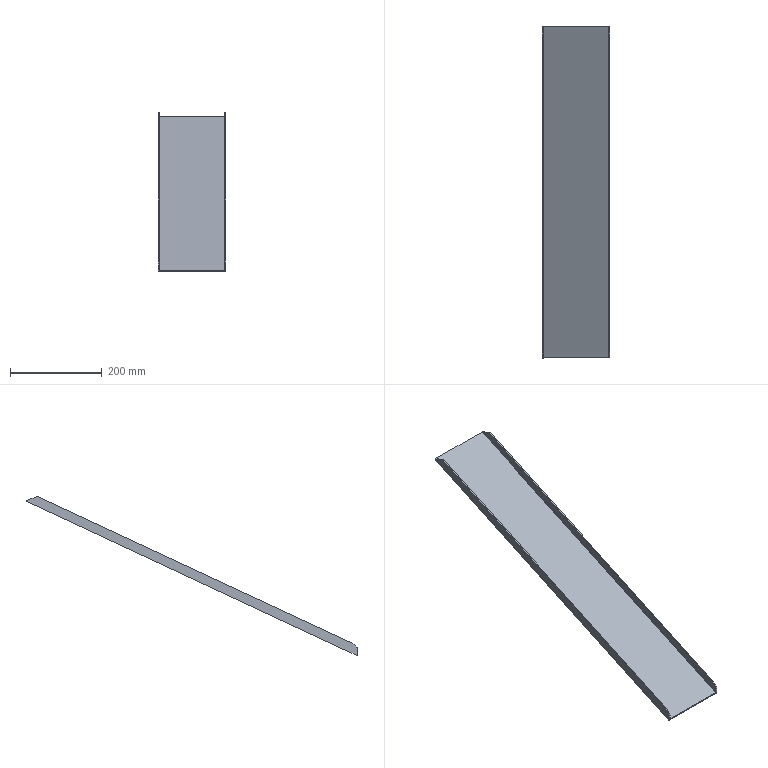Part | NX | features solid 2 | 1 solid | 16 faces | box 146.416 x 724.221 x 347.355 mm | volume 290427 mm3 | plane 9 | spline 6 | cylinder 1 | commonest cylinder face diameters 40 x1
STEP:
#1=CARTESIAN_POINT('',(-795.66,-820.,-476.696));
#2=VERTEX_POINT('',#1);
#3=CARTESIAN_POINT('',(-795.66,-820.,-478.903));
#4=VERTEX_POINT('',#3);
#5=CARTESIAN_POINT('',(-795.66,-820.,-476.696));
#6=CARTESIAN_POINT('',(-795.66,-820.,-477.432));
#7=CARTESIAN_POINT('',(-795.66,-820.,-478.167));
#8=CARTESIAN_POINT('',(-795.66,-820.,-478.902));
#9=B_SPLINE_CURVE_WITH_KNOTS('',3,(#5,#6,#7,#8),.UNSPECIFIED.,.F.,.F.,(4,4),(0.,0.002206),.UNSPECIFIED.);
#10=EDGE_CURVE('',#2,#4,#9,.T.);
#11=ORIENTED_EDGE('',*,*,#10,.F.);
#12=CARTESIAN_POINT('',(-938.,-820.,-476.696));
#13=VERTEX_POINT('',#12);
#14=CARTESIAN_POINT('',(-793.584,-820.,-476.696));
#15=DIRECTION('',(1.,0.,0.));
#16=VECTOR('',#15,1000.);
#17=LINE('',#14,#16);
#18=EDGE_CURVE('',#13,#2,#17,.T.);
#19=ORIENTED_EDGE('',*,*,#18,.F.);
#20=CARTESIAN_POINT('',(-938.,-820.,-478.903));
#21=VERTEX_POINT('',#20);
#22=CARTESIAN_POINT('',(-938.,-820.,-700.));
#23=DIRECTION('',(0.,0.,1.));
#24=VECTOR('',#23,1000.);
#25=LINE('',#22,#24);
#26=EDGE_CURVE('',#21,#13,#25,.T.);
#27=ORIENTED_EDGE('',*,*,#26,.F.);
#28=CARTESIAN_POINT('',(-793.584,-820.,-478.903));
#29=DIRECTION('',(1.,0.,0.));
#30=VECTOR('',#29,1000.);
#31=LINE('',#28,#30);
#32=EDGE_CURVE('',#21,#4,#31,.T.);
#33=ORIENTED_EDGE('',*,*,#32,.T.);
#34=EDGE_LOOP('',(#11,#19,#27,#33));
#35=FACE_BOUND('',#34,.T.);
#36=CARTESIAN_POINT('',(1065.,-820.,-700.));
#37=DIRECTION('',(0.,1.,0.));
#38=DIRECTION('',(-1.,0.,0.));
#39=AXIS2_PLACEMENT_3D('',#36,#37,#38);
#40=PLANE('',#39);
#41=ADVANCED_FACE('',(#35),#40,.F.);
#42=CARTESIAN_POINT('',(-795.584,-98.498,-140.255));
#43=VERTEX_POINT('',#42);
#44=CARTESIAN_POINT('',(-795.584,-98.499,-140.255));
#45=CARTESIAN_POINT('',(-795.661,-218.749,-196.329));
#46=CARTESIAN_POINT('',(-795.552,-459.25,-308.476));
#47=CARTESIAN_POINT('',(-795.635,-699.75,-420.623));
#48=CARTESIAN_POINT('',(-795.66,-820.,-476.696));
#49=B_SPLINE_CURVE_WITH_KNOTS('',3,(#44,#45,#46,#47,#48),.UNSPECIFIED.,.F.,.F.,(4,1,4),(0.,0.398,0.7961),.UNSPECIFIED.);
#50=EDGE_CURVE('',#43,#2,#49,.T.);
#51=ORIENTED_EDGE('',*,*,#50,.F.);
#52=CARTESIAN_POINT('',(-938.,-98.499,-140.255));
#53=VERTEX_POINT('',#52);
#54=CARTESIAN_POINT('',(-793.584,-98.499,-140.255));
#55=DIRECTION('',(-1.,0.,0.));
#56=VECTOR('',#55,1000.);
#57=LINE('',#54,#56);
#58=EDGE_CURVE('',#43,#53,#57,.T.);
#59=ORIENTED_EDGE('',*,*,#58,.T.);
#60=CARTESIAN_POINT('',(-938.,-996.354,-558.932));
#61=DIRECTION('',(0.,0.9063,0.4226));
#62=VECTOR('',#61,1000.);
#63=LINE('',#60,#62);
#64=EDGE_CURVE('',#13,#53,#63,.T.);
#65=ORIENTED_EDGE('',*,*,#64,.F.);
#66=ORIENTED_EDGE('',*,*,#18,.T.);
#67=EDGE_LOOP('',(#51,#59,#65,#66));
#68=FACE_BOUND('',#67,.T.);
#69=CARTESIAN_POINT('',(-793.584,-996.354,-558.932));
#70=DIRECTION('',(0.,0.4226,-0.9063));
#71=DIRECTION('',(-1.,0.,0.));
#72=AXIS2_PLACEMENT_3D('',#69,#70,#71);
#73=PLANE('',#72);
#74=ADVANCED_FACE('',(#68),#73,.F.);
#75=CARTESIAN_POINT('',(-795.584,-97.653,-142.067));
#76=VERTEX_POINT('',#75);
#77=CARTESIAN_POINT('',(-795.584,-97.654,-142.068));
#78=CARTESIAN_POINT('',(-795.584,-97.936,-141.463));
#79=CARTESIAN_POINT('',(-795.584,-98.217,-140.859));
#80=CARTESIAN_POINT('',(-795.584,-98.499,-140.255));
#81=B_SPLINE_CURVE_WITH_KNOTS('',3,(#77,#78,#79,#80),.UNSPECIFIED.,.F.,.F.,(4,4),(0.,1.),.UNSPECIFIED.);
#82=EDGE_CURVE('',#76,#43,#81,.T.);
#83=ORIENTED_EDGE('',*,*,#82,.F.);
#84=CARTESIAN_POINT('',(-940.,-97.654,-142.068));
#85=VERTEX_POINT('',#84);
#86=CARTESIAN_POINT('',(-793.584,-97.654,-142.068));
#87=DIRECTION('',(-1.,0.,0.));
#88=VECTOR('',#87,1000.);
#89=LINE('',#86,#88);
#90=EDGE_CURVE('',#76,#85,#89,.T.);
#91=ORIENTED_EDGE('',*,*,#90,.T.);
#92=CARTESIAN_POINT('',(-940.,-98.499,-140.255));
#93=VERTEX_POINT('',#92);
#94=CARTESIAN_POINT('',(-940.,-98.499,-140.255));
#95=DIRECTION('',(0.,0.4226,-0.9063));
#96=VECTOR('',#95,1000.);
#97=LINE('',#94,#96);
#98=EDGE_CURVE('',#93,#85,#97,.T.);
#99=ORIENTED_EDGE('',*,*,#98,.F.);
#100=CARTESIAN_POINT('',(-940.,-98.499,-140.255));
#101=DIRECTION('',(-1.,0.,0.));
#102=VECTOR('',#101,1000.);
#103=LINE('',#100,#102);
#104=EDGE_CURVE('',#93,#53,#103,.F.);
#105=ORIENTED_EDGE('',*,*,#104,.T.);
#106=ORIENTED_EDGE('',*,*,#58,.F.);
#107=EDGE_LOOP('',(#83,#91,#99,#105,#106));
#108=FACE_BOUND('',#107,.T.);
#109=CARTESIAN_POINT('',(-793.584,-98.499,-140.255));
#110=DIRECTION('',(0.,-0.9063,-0.4226));
#111=DIRECTION('',(0.,0.4226,-0.9063));
#112=AXIS2_PLACEMENT_3D('',#109,#110,#111);
#113=PLANE('',#112);
#114=ADVANCED_FACE('',(#108),#113,.F.);
#115=CARTESIAN_POINT('',(-793.66,-820.,-478.903));
#116=VERTEX_POINT('',#115);
#117=CARTESIAN_POINT('',(-793.584,-97.654,-142.068));
#118=VERTEX_POINT('',#117);
#119=CARTESIAN_POINT('',(-793.66,-820.,-478.903));
#120=CARTESIAN_POINT('',(-793.635,-699.609,-422.764));
#121=CARTESIAN_POINT('',(-793.552,-458.827,-310.485));
#122=CARTESIAN_POINT('',(-793.661,-218.045,-198.207));
#123=CARTESIAN_POINT('',(-793.584,-97.654,-142.068));
#124=B_SPLINE_CURVE_WITH_KNOTS('',3,(#119,#120,#121,#122,#123),.UNSPECIFIED.,.F.,.F.,(4,1,4),(0.,0.3985,0.797),.UNSPECIFIED.);
#125=EDGE_CURVE('',#116,#118,#124,.T.);
#126=ORIENTED_EDGE('',*,*,#125,.T.);
#127=CARTESIAN_POINT('',(-793.584,-98.499,-140.255));
#128=VERTEX_POINT('',#127);
#129=CARTESIAN_POINT('',(-793.584,-98.499,-140.255));
#130=CARTESIAN_POINT('',(-793.584,-98.217,-140.859));
#131=CARTESIAN_POINT('',(-793.584,-97.936,-141.463));
#132=CARTESIAN_POINT('',(-793.584,-97.654,-142.068));
#133=B_SPLINE_CURVE_WITH_KNOTS('',3,(#129,#130,#131,#132),.UNSPECIFIED.,.F.,.F.,(4,4),(0.,1.),.UNSPECIFIED.);
#134=EDGE_CURVE('',#118,#128,#133,.F.);
#135=ORIENTED_EDGE('',*,*,#134,.T.);
#136=CARTESIAN_POINT('',(-793.66,-820.,-476.696));
#137=VERTEX_POINT('',#136);
#138=CARTESIAN_POINT('',(-793.584,-98.499,-140.255));
#139=CARTESIAN_POINT('',(-793.586,-101.89,-141.836));
#140=CARTESIAN_POINT('',(-793.59,-108.28,-144.816));
#141=CARTESIAN_POINT('',(-793.595,-116.688,-148.736));
#142=CARTESIAN_POINT('',(-793.6,-123.917,-152.107));
#143=CARTESIAN_POINT('',(-793.603,-129.968,-154.929));
#144=CARTESIAN_POINT('',(-793.605,-134.029,-156.823));
#145=CARTESIAN_POINT('',(-793.607,-136.689,-158.063));
#146=CARTESIAN_POINT('',(-793.608,-138.389,-158.856));
#147=CARTESIAN_POINT('',(-793.608,-139.561,-159.402));
#148=CARTESIAN_POINT('',(-793.609,-140.351,-159.771));
#149=CARTESIAN_POINT('',(-793.609,-140.87,-160.013));
#150=CARTESIAN_POINT('',(-793.609,-141.315,-160.22));
#151=CARTESIAN_POINT('',(-793.609,-141.625,-160.365));
#152=CARTESIAN_POINT('',(-793.609,-141.835,-160.463));
#153=CARTESIAN_POINT('',(-793.609,-141.976,-160.528));
#154=CARTESIAN_POINT('',(-793.609,-142.076,-160.575));
#155=CARTESIAN_POINT('',(-793.609,-142.15,-160.609));
#156=CARTESIAN_POINT('',(-793.609,-142.185,-160.626));
#157=CARTESIAN_POINT('',(-793.609,-142.226,-160.645));
#158=CARTESIAN_POINT('',(-793.609,-142.216,-160.641));
#159=CARTESIAN_POINT('',(-793.609,-142.642,-160.839));
#160=CARTESIAN_POINT('',(-793.609,-143.054,-161.031));
#161=CARTESIAN_POINT('',(-793.608,-143.617,-161.294));
#162=CARTESIAN_POINT('',(-793.608,-144.479,-161.696));
#163=CARTESIAN_POINT('',(-793.608,-145.546,-162.193));
#164=CARTESIAN_POINT('',(-793.607,-147.207,-162.968));
#165=CARTESIAN_POINT('',(-793.606,-149.208,-163.901));
#166=CARTESIAN_POINT('',(-793.605,-152.244,-165.317));
#167=CARTESIAN_POINT('',(-793.603,-155.733,-166.943));
#168=CARTESIAN_POINT('',(-793.602,-159.426,-168.665));
#169=CARTESIAN_POINT('',(-793.601,-162.626,-170.158));
#170=CARTESIAN_POINT('',(-793.6,-165.334,-171.421));
#171=CARTESIAN_POINT('',(-793.599,-167.549,-172.454));
#172=CARTESIAN_POINT('',(-793.598,-169.272,-173.257));
#173=CARTESIAN_POINT('',(-793.598,-170.297,-173.735));
#174=CARTESIAN_POINT('',(-793.598,-170.871,-174.003));
#175=CARTESIAN_POINT('',(-793.598,-171.176,-174.145));
#176=CARTESIAN_POINT('',(-793.598,-171.321,-174.213));
#177=CARTESIAN_POINT('',(-793.598,-171.365,-174.233));
#178=CARTESIAN_POINT('',(-793.598,-171.406,-174.252));
#179=CARTESIAN_POINT('',(-793.597,-171.346,-174.224));
#180=CARTESIAN_POINT('',(-793.598,-171.617,-174.35));
#181=CARTESIAN_POINT('',(-793.598,-171.941,-174.501));
#182=CARTESIAN_POINT('',(-793.599,-172.461,-174.744));
#183=CARTESIAN_POINT('',(-793.6,-173.361,-175.164));
#184=CARTESIAN_POINT('',(-793.601,-174.494,-175.692));
#185=CARTESIAN_POINT('',(-793.602,-175.851,-176.325));
#186=CARTESIAN_POINT('',(-793.603,-177.66,-177.168));
#187=CARTESIAN_POINT('',(-793.605,-179.922,-178.223));
#188=CARTESIAN_POINT('',(-793.606,-182.636,-179.489));
#189=CARTESIAN_POINT('',(-793.608,-186.255,-181.176));
#190=CARTESIAN_POINT('',(-793.609,-189.874,-182.864));
#191=CARTESIAN_POINT('',(-793.609,-193.492,-184.551));
#192=CARTESIAN_POINT('',(-793.608,-195.754,-185.606));
#193=CARTESIAN_POINT('',(-793.608,-197.563,-186.449));
#194=CARTESIAN_POINT('',(-793.607,-198.696,-186.977));
#195=CARTESIAN_POINT('',(-793.607,-199.484,-187.345));
#196=CARTESIAN_POINT('',(-793.607,-199.941,-187.558));
#197=CARTESIAN_POINT('',(-793.607,-200.267,-187.71));
#198=CARTESIAN_POINT('',(-793.606,-200.592,-187.862));
#199=CARTESIAN_POINT('',(-793.606,-200.551,-187.843));
#200=CARTESIAN_POINT('',(-793.606,-200.568,-187.851));
#201=CARTESIAN_POINT('',(-793.606,-200.563,-187.848));
#202=CARTESIAN_POINT('',(-793.606,-200.596,-187.863));
#203=CARTESIAN_POINT('',(-793.606,-200.64,-187.884));
#204=CARTESIAN_POINT('',(-793.606,-200.706,-187.915));
#205=CARTESIAN_POINT('',(-793.606,-200.817,-187.967));
#206=CARTESIAN_POINT('',(-793.606,-201.001,-188.052));
#207=CARTESIAN_POINT('',(-793.606,-201.293,-188.188));
#208=CARTESIAN_POINT('',(-793.606,-201.657,-188.358));
#209=CARTESIAN_POINT('',(-793.606,-202.238,-188.629));
#210=CARTESIAN_POINT('',(-793.606,-203.144,-189.052));
#211=CARTESIAN_POINT('',(-793.606,-204.977,-189.906));
#212=CARTESIAN_POINT('',(-793.606,-207.987,-191.31));
#213=CARTESIAN_POINT('',(-793.606,-212.748,-193.53));
#214=CARTESIAN_POINT('',(-793.606,-218.659,-196.286));
#215=CARTESIAN_POINT('',(-793.605,-225.72,-199.579));
#216=CARTESIAN_POINT('',(-793.605,-233.93,-203.408));
#217=CARTESIAN_POINT('',(-793.605,-246.41,-209.227));
#218=CARTESIAN_POINT('',(-793.604,-261.19,-216.119));
#219=CARTESIAN_POINT('',(-793.604,-278.269,-224.083));
#220=CARTESIAN_POINT('',(-793.603,-292.228,-230.592));
#221=CARTESIAN_POINT('',(-793.603,-307.337,-237.637));
#222=CARTESIAN_POINT('',(-793.602,-323.595,-245.219));
#223=CARTESIAN_POINT('',(-793.602,-338.102,-251.983));
#224=CARTESIAN_POINT('',(-793.601,-350.282,-257.663));
#225=CARTESIAN_POINT('',(-793.601,-359.704,-262.057));
#226=CARTESIAN_POINT('',(-793.6,-369.414,-266.585));
#227=CARTESIAN_POINT('',(-793.6,-377.745,-270.47));
#228=CARTESIAN_POINT('',(-793.6,-384.554,-273.645));
#229=CARTESIAN_POINT('',(-793.6,-389.732,-276.059));
#230=CARTESIAN_POINT('',(-793.6,-394.107,-278.099));
#231=CARTESIAN_POINT('',(-793.6,-397.644,-279.749));
#232=CARTESIAN_POINT('',(-793.599,-399.868,-280.785));
#233=CARTESIAN_POINT('',(-793.599,-401.659,-281.621));
#234=CARTESIAN_POINT('',(-793.599,-402.775,-282.141));
#235=CARTESIAN_POINT('',(-793.599,-403.687,-282.567));
#236=CARTESIAN_POINT('',(-793.599,-404.218,-282.814));
#237=CARTESIAN_POINT('',(-793.599,-404.736,-283.056));
#238=CARTESIAN_POINT('',(-793.599,-404.8,-283.085));
#239=CARTESIAN_POINT('',(-793.599,-405.124,-283.236));
#240=CARTESIAN_POINT('',(-793.599,-405.476,-283.401));
#241=CARTESIAN_POINT('',(-793.599,-406.103,-283.693));
#242=CARTESIAN_POINT('',(-793.599,-406.868,-284.05));
#243=CARTESIAN_POINT('',(-793.599,-407.799,-284.484));
#244=CARTESIAN_POINT('',(-793.599,-409.042,-285.064));
#245=CARTESIAN_POINT('',(-793.599,-411.233,-286.085));
#246=CARTESIAN_POINT('',(-793.599,-414.401,-287.562));
#247=CARTESIAN_POINT('',(-793.599,-418.265,-289.364));
#248=CARTESIAN_POINT('',(-793.599,-422.191,-291.195));
#249=CARTESIAN_POINT('',(-793.599,-427.509,-293.675));
#250=CARTESIAN_POINT('',(-793.599,-434.313,-296.847));
#251=CARTESIAN_POINT('',(-793.599,-442.726,-300.771));
#252=CARTESIAN_POINT('',(-793.6,-454.276,-306.157));
#253=CARTESIAN_POINT('',(-793.601,-469.337,-313.179));
#254=CARTESIAN_POINT('',(-793.602,-488.406,-322.072));
#255=CARTESIAN_POINT('',(-793.604,-508.473,-331.429));
#256=CARTESIAN_POINT('',(-793.607,-529.536,-341.251));
#257=CARTESIAN_POINT('',(-793.61,-558.949,-354.966));
#258=CARTESIAN_POINT('',(-793.616,-598.208,-373.273));
#259=CARTESIAN_POINT('',(-793.624,-640.79,-393.129));
#260=CARTESIAN_POINT('',(-793.631,-676.85,-409.944));
#261=CARTESIAN_POINT('',(-793.635,-700.215,-420.84));
#262=CARTESIAN_POINT('',(-793.639,-719.412,-429.791));
#263=CARTESIAN_POINT('',(-793.643,-738.564,-438.722));
#264=CARTESIAN_POINT('',(-793.648,-762.519,-449.893));
#265=CARTESIAN_POINT('',(-793.654,-791.259,-463.294));
#266=CARTESIAN_POINT('',(-793.658,-810.42,-472.229));
#267=CARTESIAN_POINT('',(-793.66,-820.,-476.696));
#268=B_SPLINE_CURVE_WITH_KNOTS('',3,(#138,#139,#140,#141,#142,#143,#144,#145,#146,#147,#148,#149,#150,#151,#152,#153,#154,#155,#156,#157,#158,#159,#160,#161,#162,#163,#164,#165,#166,#167,#168,#169,#170,#171,#172,#173,#174,#175,#176,#177,#178,#179,#180,#181,#182,#183,#184,#185,#186,#187,#188,#189,#190,#191,#192,#193,#194,#195,#196,#197,#198,#199,#200,#201,#202,#203,#204,#205,#206,#207,#208,#209,#210,#211,#212,#213,#214,#215,#216,#217,#218,#219,#220,#221,#222,#223,#224,#225,#226,#227,#228,#229,#230,#231,#232,#233,#234,#235,#236,#237,#238,#239,#240,#241,#242,#243,#244,#245,#246,#247,#248,#249,#250,#251,#252,#253,#254,#255,#256,#257,#258,#259,#260,#261,#262,#263,#264,#265,#266,#267),.UNSPECIFIED.,.F.,.F.,(4,1,1,1,1,1,1,1,1,1,1,1,1,1,1,1,1,1,1,1,1,1,1,1,1,1,1,1,1,1,1,1,1,1,1,1,1,1,1,1,1,1,1,1,1,1,1,1,1,1,1,1,1,1,1,1,1,1,1,1,1,1,1,1,1,1,1,1,1,1,1,1,1,1,1,1,1,1,1,1,1,1,1,1,1,1,1,1,1,1,1,1,1,1,1,1,1,1,1,1,1,1,1,1,1,1,1,1,1,1,1,1,1,1,1,1,1,1,1,1,1,1,1,1,1,1,1,4),(0.,0.008865,0.01773,0.02659,0.03546,0.04432,0.04876,0.05319,0.05762,0.05984,0.06205,0.06427,0.06648,0.06759,0.0687,0.06981,0.07036,0.07092,0.07119,0.07147,0.07175,0.07202,0.07258,0.07313,0.07424,0.07535,0.07757,0.07978,0.08421,0.08865,0.09308,0.09751,0.1019,0.1064,0.1108,0.113,0.1152,0.1175,0.118,0.1186,0.1191,0.1194,0.1197,0.1208,0.1219,0.1241,0.1263,0.1285,0.133,0.1374,0.1418,0.1507,0.1551,0.1596,0.1618,0.164,0.1651,0.1657,0.1662,0.1668,0.167,0.1673,0.1684,0.1706,0.1729,0.1751,0.1773,0.1817,0.1862,0.1906,0.195,0.2039,0.2127,0.2305,0.2482,0.2659,0.2837,0.3014,0.3191,0.3546,0.3723,0.39,0.4078,0.4255,0.4432,0.4521,0.461,0.4698,0.4787,0.4831,0.4876,0.492,0.4942,0.4964,0.4975,0.4986,0.4992,0.4997,0.5,0.5003,0.5008,0.502,0.5031,0.5053,0.5075,0.5097,0.5141,0.523,0.5319,0.5407,0.5496,0.5673,0.5851,0.6028,0.6382,0.6737,0.7092,0.7446,0.7801,0.851,0.9219,0.9574,0.9928,1.011,1.028,1.064,1.099,1.135),.UNSPECIFIED.);
#269=EDGE_CURVE('',#128,#137,#268,.T.);
#270=ORIENTED_EDGE('',*,*,#269,.T.);
#271=CARTESIAN_POINT('',(-793.66,-820.,-476.696));
#272=CARTESIAN_POINT('',(-793.66,-820.,-477.432));
#273=CARTESIAN_POINT('',(-793.66,-820.,-478.168));
#274=CARTESIAN_POINT('',(-793.66,-820.,-478.903));
#275=B_SPLINE_CURVE_WITH_KNOTS('',3,(#271,#272,#273,#274),.UNSPECIFIED.,.F.,.F.,(4,4),(0.,1.),.UNSPECIFIED.);
#276=EDGE_CURVE('',#137,#116,#275,.T.);
#277=ORIENTED_EDGE('',*,*,#276,.T.);
#278=EDGE_LOOP('',(#126,#135,#270,#277));
#279=FACE_BOUND('',#278,.T.);
#280=CARTESIAN_POINT('',(-793.661,-826.369,-479.666));
#281=CARTESIAN_POINT('',(-793.661,-825.523,-481.479));
#282=CARTESIAN_POINT('',(-793.657,-807.075,-470.669));
#283=CARTESIAN_POINT('',(-793.657,-806.23,-472.482));
#284=CARTESIAN_POINT('',(-793.651,-778.138,-457.176));
#285=CARTESIAN_POINT('',(-793.651,-777.292,-458.988));
#286=CARTESIAN_POINT('',(-793.644,-744.368,-441.429));
#287=CARTESIAN_POINT('',(-793.644,-743.523,-443.241));
#288=CARTESIAN_POINT('',(-793.64,-725.084,-432.436));
#289=CARTESIAN_POINT('',(-793.64,-724.239,-434.249));
#290=CARTESIAN_POINT('',(-793.637,-710.586,-425.676));
#291=CARTESIAN_POINT('',(-793.637,-709.741,-427.488));
#292=CARTESIAN_POINT('',(-793.634,-696.222,-418.978));
#293=CARTESIAN_POINT('',(-793.634,-695.376,-420.79));
#294=CARTESIAN_POINT('',(-793.631,-677.447,-410.223));
#295=CARTESIAN_POINT('',(-793.631,-676.602,-412.036));
#296=CARTESIAN_POINT('',(-793.626,-654.597,-399.568));
#297=CARTESIAN_POINT('',(-793.626,-653.752,-401.38));
#298=CARTESIAN_POINT('',(-793.622,-628.193,-387.255));
#299=CARTESIAN_POINT('',(-793.622,-627.348,-389.068));
#300=CARTESIAN_POINT('',(-793.617,-602.798,-375.414));
#301=CARTESIAN_POINT('',(-793.617,-601.953,-377.226));
#302=CARTESIAN_POINT('',(-793.613,-578.415,-364.043));
#303=CARTESIAN_POINT('',(-793.613,-577.57,-365.856));
#304=CARTESIAN_POINT('',(-793.61,-555.042,-353.144));
#305=CARTESIAN_POINT('',(-793.61,-554.197,-354.957));
#306=CARTESIAN_POINT('',(-793.607,-532.68,-342.717));
#307=CARTESIAN_POINT('',(-793.607,-531.834,-344.529));
#308=CARTESIAN_POINT('',(-793.604,-511.328,-332.76));
#309=CARTESIAN_POINT('',(-793.604,-510.483,-334.573));
#310=CARTESIAN_POINT('',(-793.602,-490.987,-323.275));
#311=CARTESIAN_POINT('',(-793.602,-490.142,-325.088));
#312=CARTESIAN_POINT('',(-793.601,-474.879,-315.764));
#313=CARTESIAN_POINT('',(-793.601,-474.033,-317.576));
#314=CARTESIAN_POINT('',(-793.6,-462.497,-309.99));
#315=CARTESIAN_POINT('',(-793.6,-461.652,-311.803));
#316=CARTESIAN_POINT('',(-793.6,-453.464,-305.778));
#317=CARTESIAN_POINT('',(-793.6,-452.619,-307.59));
#318=CARTESIAN_POINT('',(-793.599,-444.683,-301.683));
#319=CARTESIAN_POINT('',(-793.599,-443.838,-303.496));
#320=CARTESIAN_POINT('',(-793.599,-436.155,-297.707));
#321=CARTESIAN_POINT('',(-793.599,-435.31,-299.519));
#322=CARTESIAN_POINT('',(-793.599,-429.259,-294.491));
#323=CARTESIAN_POINT('',(-793.599,-428.414,-296.303));
#324=CARTESIAN_POINT('',(-793.599,-423.868,-291.977));
#325=CARTESIAN_POINT('',(-793.599,-423.023,-293.79));
#326=CARTESIAN_POINT('',(-793.599,-419.889,-290.121));
#327=CARTESIAN_POINT('',(-793.599,-419.043,-291.934));
#328=CARTESIAN_POINT('',(-793.599,-416.625,-288.599));
#329=CARTESIAN_POINT('',(-793.599,-415.779,-290.412));
#330=CARTESIAN_POINT('',(-793.599,-414.045,-287.397));
#331=CARTESIAN_POINT('',(-793.599,-413.2,-289.209));
#332=CARTESIAN_POINT('',(-793.599,-412.126,-286.502));
#333=CARTESIAN_POINT('',(-793.599,-411.281,-288.314));
#334=CARTESIAN_POINT('',(-793.599,-410.223,-285.614));
#335=CARTESIAN_POINT('',(-793.599,-409.378,-287.427));
#336=CARTESIAN_POINT('',(-793.599,-408.651,-284.881));
#337=CARTESIAN_POINT('',(-793.599,-407.805,-286.694));
#338=CARTESIAN_POINT('',(-793.599,-407.4,-284.298));
#339=CARTESIAN_POINT('',(-793.599,-406.555,-286.111));
#340=CARTESIAN_POINT('',(-793.599,-406.623,-283.935));
#341=CARTESIAN_POINT('',(-793.599,-405.777,-285.748));
#342=CARTESIAN_POINT('',(-793.599,-406.001,-283.646));
#343=CARTESIAN_POINT('',(-793.599,-405.156,-285.458));
#344=CARTESIAN_POINT('',(-793.599,-405.54,-283.43));
#345=CARTESIAN_POINT('',(-793.599,-404.694,-285.243));
#346=CARTESIAN_POINT('',(-793.599,-405.144,-283.246));
#347=CARTESIAN_POINT('',(-793.599,-404.299,-285.059));
#348=CARTESIAN_POINT('',(-793.599,-404.891,-283.128));
#349=CARTESIAN_POINT('',(-793.599,-404.046,-284.94));
#350=CARTESIAN_POINT('',(-793.599,-404.733,-283.054));
#351=CARTESIAN_POINT('',(-793.599,-403.888,-284.867));
#352=CARTESIAN_POINT('',(-793.599,-404.693,-283.036));
#353=CARTESIAN_POINT('',(-793.599,-403.848,-284.848));
#354=CARTESIAN_POINT('',(-793.599,-404.42,-282.908));
#355=CARTESIAN_POINT('',(-793.599,-403.575,-284.721));
#356=CARTESIAN_POINT('',(-793.599,-404.159,-282.786));
#357=CARTESIAN_POINT('',(-793.599,-403.313,-284.599));
#358=CARTESIAN_POINT('',(-793.599,-403.696,-282.571));
#359=CARTESIAN_POINT('',(-793.599,-402.851,-284.383));
#360=CARTESIAN_POINT('',(-793.599,-402.909,-282.203));
#361=CARTESIAN_POINT('',(-793.599,-402.063,-284.016));
#362=CARTESIAN_POINT('',(-793.599,-401.776,-281.675));
#363=CARTESIAN_POINT('',(-793.599,-400.93,-283.488));
#364=CARTESIAN_POINT('',(-793.599,-400.425,-281.045));
#365=CARTESIAN_POINT('',(-793.599,-399.58,-282.858));
#366=CARTESIAN_POINT('',(-793.599,-398.629,-280.208));
#367=CARTESIAN_POINT('',(-793.599,-397.784,-282.02));
#368=CARTESIAN_POINT('',(-793.6,-396.396,-279.166));
#369=CARTESIAN_POINT('',(-793.6,-395.551,-280.979));
#370=CARTESIAN_POINT('',(-793.6,-392.847,-277.511));
#371=CARTESIAN_POINT('',(-793.6,-392.001,-279.324));
#372=CARTESIAN_POINT('',(-793.6,-388.456,-275.464));
#373=CARTESIAN_POINT('',(-793.6,-387.611,-277.277));
#374=CARTESIAN_POINT('',(-793.6,-383.26,-273.041));
#375=CARTESIAN_POINT('',(-793.6,-382.414,-274.854));
#376=CARTESIAN_POINT('',(-793.6,-378.136,-270.652));
#377=CARTESIAN_POINT('',(-793.6,-377.291,-272.465));
#378=CARTESIAN_POINT('',(-793.6,-371.402,-267.512));
#379=CARTESIAN_POINT('',(-793.6,-370.557,-269.324));
#380=CARTESIAN_POINT('',(-793.601,-363.167,-263.672));
#381=CARTESIAN_POINT('',(-793.601,-362.322,-265.484));
#382=CARTESIAN_POINT('',(-793.601,-353.576,-259.199));
#383=CARTESIAN_POINT('',(-793.601,-352.731,-261.012));
#384=CARTESIAN_POINT('',(-793.601,-344.276,-254.863));
#385=CARTESIAN_POINT('',(-793.601,-343.431,-256.675));
#386=CARTESIAN_POINT('',(-793.602,-335.268,-250.662));
#387=CARTESIAN_POINT('',(-793.602,-334.423,-252.475));
#388=CARTESIAN_POINT('',(-793.602,-323.646,-245.243));
#389=CARTESIAN_POINT('',(-793.602,-322.8,-247.055));
#390=CARTESIAN_POINT('',(-793.602,-309.846,-238.808));
#391=CARTESIAN_POINT('',(-793.602,-309.001,-240.62));
#392=CARTESIAN_POINT('',(-793.603,-294.453,-231.63));
#393=CARTESIAN_POINT('',(-793.603,-293.607,-233.442));
#394=CARTESIAN_POINT('',(-793.604,-280.225,-224.995));
#395=CARTESIAN_POINT('',(-793.604,-279.38,-226.808));
#396=CARTESIAN_POINT('',(-793.604,-262.808,-216.874));
#397=CARTESIAN_POINT('',(-793.604,-261.963,-218.686));
#398=CARTESIAN_POINT('',(-793.605,-247.723,-209.839));
#399=CARTESIAN_POINT('',(-793.605,-246.878,-211.652));
#400=CARTESIAN_POINT('',(-793.605,-234.97,-203.892));
#401=CARTESIAN_POINT('',(-793.605,-234.124,-205.705));
#402=CARTESIAN_POINT('',(-793.605,-226.57,-199.975));
#403=CARTESIAN_POINT('',(-793.605,-225.725,-201.788));
#404=CARTESIAN_POINT('',(-793.606,-219.336,-196.602));
#405=CARTESIAN_POINT('',(-793.606,-218.491,-198.415));
#406=CARTESIAN_POINT('',(-793.606,-213.268,-193.773));
#407=CARTESIAN_POINT('',(-793.606,-212.423,-195.585));
#408=CARTESIAN_POINT('',(-793.606,-208.365,-191.486));
#409=CARTESIAN_POINT('',(-793.606,-207.52,-193.299));
#410=CARTESIAN_POINT('',(-793.606,-205.251,-190.034));
#411=CARTESIAN_POINT('',(-793.606,-204.406,-191.847));
#412=CARTESIAN_POINT('',(-793.606,-203.343,-189.144));
#413=CARTESIAN_POINT('',(-793.606,-202.498,-190.957));
#414=CARTESIAN_POINT('',(-793.606,-202.203,-188.613));
#415=CARTESIAN_POINT('',(-793.606,-201.358,-190.426));
#416=CARTESIAN_POINT('',(-793.606,-201.496,-188.283));
#417=CARTESIAN_POINT('',(-793.606,-200.651,-190.096));
#418=CARTESIAN_POINT('',(-793.606,-201.076,-188.087));
#419=CARTESIAN_POINT('',(-793.606,-200.231,-189.9));
#420=CARTESIAN_POINT('',(-793.606,-200.834,-187.974));
#421=CARTESIAN_POINT('',(-793.606,-199.988,-189.787));
#422=CARTESIAN_POINT('',(-793.606,-200.694,-187.909));
#423=CARTESIAN_POINT('',(-793.606,-199.848,-189.722));
#424=CARTESIAN_POINT('',(-793.606,-200.615,-187.872));
#425=CARTESIAN_POINT('',(-793.606,-199.77,-189.685));
#426=CARTESIAN_POINT('',(-793.606,-200.588,-187.86));
#427=CARTESIAN_POINT('',(-793.606,-199.743,-189.672));
#428=CARTESIAN_POINT('',(-793.606,-200.56,-187.847));
#429=CARTESIAN_POINT('',(-793.606,-199.715,-189.659));
#430=CARTESIAN_POINT('',(-793.606,-200.581,-187.857));
#431=CARTESIAN_POINT('',(-793.606,-199.736,-189.669));
#432=CARTESIAN_POINT('',(-793.606,-200.532,-187.834));
#433=CARTESIAN_POINT('',(-793.606,-199.687,-189.646));
#434=CARTESIAN_POINT('',(-793.606,-200.578,-187.855));
#435=CARTESIAN_POINT('',(-793.606,-199.733,-189.668));
#436=CARTESIAN_POINT('',(-793.606,-200.429,-187.786));
#437=CARTESIAN_POINT('',(-793.606,-199.583,-189.598));
#438=CARTESIAN_POINT('',(-793.607,-200.251,-187.703));
#439=CARTESIAN_POINT('',(-793.607,-199.406,-189.515));
#440=CARTESIAN_POINT('',(-793.607,-199.955,-187.564));
#441=CARTESIAN_POINT('',(-793.607,-199.109,-189.377));
#442=CARTESIAN_POINT('',(-793.607,-199.278,-187.249));
#443=CARTESIAN_POINT('',(-793.607,-198.433,-189.062));
#444=CARTESIAN_POINT('',(-793.607,-198.248,-186.769));
#445=CARTESIAN_POINT('',(-793.607,-197.403,-188.581));
#446=CARTESIAN_POINT('',(-793.608,-196.883,-186.132));
#447=CARTESIAN_POINT('',(-793.608,-196.038,-187.945));
#448=CARTESIAN_POINT('',(-793.608,-195.517,-185.495));
#449=CARTESIAN_POINT('',(-793.608,-194.671,-187.308));
#450=CARTESIAN_POINT('',(-793.608,-193.695,-184.645));
#451=CARTESIAN_POINT('',(-793.608,-192.849,-186.458));
#452=CARTESIAN_POINT('',(-793.609,-191.417,-183.583));
#453=CARTESIAN_POINT('',(-793.609,-190.572,-185.396));
#454=CARTESIAN_POINT('',(-793.608,-188.684,-182.309));
#455=CARTESIAN_POINT('',(-793.608,-187.839,-184.122));
#456=CARTESIAN_POINT('',(-793.608,-185.951,-181.035));
#457=CARTESIAN_POINT('',(-793.608,-185.106,-182.847));
#458=CARTESIAN_POINT('',(-793.607,-183.219,-179.76));
#459=CARTESIAN_POINT('',(-793.607,-182.373,-181.573));
#460=CARTESIAN_POINT('',(-793.605,-180.486,-178.486));
#461=CARTESIAN_POINT('',(-793.605,-179.64,-180.299));
#462=CARTESIAN_POINT('',(-793.604,-178.208,-177.424));
#463=CARTESIAN_POINT('',(-793.604,-177.363,-179.237));
#464=CARTESIAN_POINT('',(-793.602,-176.386,-176.574));
#465=CARTESIAN_POINT('',(-793.602,-175.541,-178.387));
#466=CARTESIAN_POINT('',(-793.601,-175.02,-175.937));
#467=CARTESIAN_POINT('',(-793.601,-174.174,-177.75));
#468=CARTESIAN_POINT('',(-793.6,-173.882,-175.407));
#469=CARTESIAN_POINT('',(-793.6,-173.037,-177.219));
#470=CARTESIAN_POINT('',(-793.599,-172.969,-174.981));
#471=CARTESIAN_POINT('',(-793.599,-172.124,-176.793));
#472=CARTESIAN_POINT('',(-793.599,-172.405,-174.718));
#473=CARTESIAN_POINT('',(-793.599,-171.559,-176.53));
#474=CARTESIAN_POINT('',(-793.598,-171.939,-174.5));
#475=CARTESIAN_POINT('',(-793.598,-171.094,-176.313));
#476=CARTESIAN_POINT('',(-793.598,-171.681,-174.38));
#477=CARTESIAN_POINT('',(-793.598,-170.835,-176.193));
#478=CARTESIAN_POINT('',(-793.598,-171.399,-174.249));
#479=CARTESIAN_POINT('',(-793.598,-170.553,-176.061));
#480=CARTESIAN_POINT('',(-793.598,-171.392,-174.246));
#481=CARTESIAN_POINT('',(-793.598,-170.547,-176.058));
#482=CARTESIAN_POINT('',(-793.598,-171.374,-174.237));
#483=CARTESIAN_POINT('',(-793.598,-170.529,-176.05));
#484=CARTESIAN_POINT('',(-793.598,-171.329,-174.216));
#485=CARTESIAN_POINT('',(-793.598,-170.483,-176.029));
#486=CARTESIAN_POINT('',(-793.598,-171.214,-174.163));
#487=CARTESIAN_POINT('',(-793.598,-170.369,-175.975));
#488=CARTESIAN_POINT('',(-793.598,-170.993,-174.06));
#489=CARTESIAN_POINT('',(-793.598,-170.148,-175.872));
#490=CARTESIAN_POINT('',(-793.598,-170.474,-173.817));
#491=CARTESIAN_POINT('',(-793.598,-169.628,-175.63));
#492=CARTESIAN_POINT('',(-793.598,-169.512,-173.369));
#493=CARTESIAN_POINT('',(-793.598,-168.666,-175.181));
#494=CARTESIAN_POINT('',(-793.599,-167.858,-172.597));
#495=CARTESIAN_POINT('',(-793.599,-167.012,-174.41));
#496=CARTESIAN_POINT('',(-793.599,-165.704,-171.593));
#497=CARTESIAN_POINT('',(-793.599,-164.859,-173.406));
#498=CARTESIAN_POINT('',(-793.601,-163.052,-170.356));
#499=CARTESIAN_POINT('',(-793.601,-162.206,-172.169));
#500=CARTESIAN_POINT('',(-793.602,-159.899,-168.886));
#501=CARTESIAN_POINT('',(-793.602,-159.054,-170.699));
#502=CARTESIAN_POINT('',(-793.603,-156.856,-167.467));
#503=CARTESIAN_POINT('',(-793.603,-156.011,-169.28));
#504=CARTESIAN_POINT('',(-793.604,-154.172,-166.216));
#505=CARTESIAN_POINT('',(-793.604,-153.327,-168.028));
#506=CARTESIAN_POINT('',(-793.605,-152.034,-165.219));
#507=CARTESIAN_POINT('',(-793.605,-151.189,-167.031));
#508=CARTESIAN_POINT('',(-793.606,-149.771,-164.164));
#509=CARTESIAN_POINT('',(-793.606,-148.926,-165.976));
#510=CARTESIAN_POINT('',(-793.607,-147.782,-163.236));
#511=CARTESIAN_POINT('',(-793.607,-146.936,-165.048));
#512=CARTESIAN_POINT('',(-793.607,-146.127,-162.464));
#513=CARTESIAN_POINT('',(-793.607,-145.282,-164.277));
#514=CARTESIAN_POINT('',(-793.608,-145.068,-161.97));
#515=CARTESIAN_POINT('',(-793.608,-144.223,-163.783));
#516=CARTESIAN_POINT('',(-793.608,-144.203,-161.567));
#517=CARTESIAN_POINT('',(-793.608,-143.357,-163.38));
#518=CARTESIAN_POINT('',(-793.608,-143.553,-161.264));
#519=CARTESIAN_POINT('',(-793.608,-142.708,-163.076));
#520=CARTESIAN_POINT('',(-793.609,-142.983,-160.998));
#521=CARTESIAN_POINT('',(-793.609,-142.137,-162.811));
#522=CARTESIAN_POINT('',(-793.609,-142.572,-160.807));
#523=CARTESIAN_POINT('',(-793.609,-141.727,-162.619));
#524=CARTESIAN_POINT('',(-793.609,-142.201,-160.634));
#525=CARTESIAN_POINT('',(-793.609,-141.356,-162.446));
#526=CARTESIAN_POINT('',(-793.609,-142.233,-160.648));
#527=CARTESIAN_POINT('',(-793.609,-141.387,-162.461));
#528=CARTESIAN_POINT('',(-793.609,-142.207,-160.636));
#529=CARTESIAN_POINT('',(-793.609,-141.361,-162.449));
#530=CARTESIAN_POINT('',(-793.609,-142.186,-160.627));
#531=CARTESIAN_POINT('',(-793.609,-141.341,-162.439));
#532=CARTESIAN_POINT('',(-793.609,-142.141,-160.605));
#533=CARTESIAN_POINT('',(-793.609,-141.295,-162.418));
#534=CARTESIAN_POINT('',(-793.609,-142.087,-160.58));
#535=CARTESIAN_POINT('',(-793.609,-141.242,-162.393));
#536=CARTESIAN_POINT('',(-793.609,-142.007,-160.543));
#537=CARTESIAN_POINT('',(-793.609,-141.162,-162.356));
#538=CARTESIAN_POINT('',(-793.609,-141.897,-160.492));
#539=CARTESIAN_POINT('',(-793.609,-141.052,-162.304));
#540=CARTESIAN_POINT('',(-793.609,-141.695,-160.397));
#541=CARTESIAN_POINT('',(-793.609,-140.85,-162.21));
#542=CARTESIAN_POINT('',(-793.609,-141.396,-160.258));
#543=CARTESIAN_POINT('',(-793.609,-140.55,-162.071));
#544=CARTESIAN_POINT('',(-793.609,-140.962,-160.056));
#545=CARTESIAN_POINT('',(-793.609,-140.117,-161.868));
#546=CARTESIAN_POINT('',(-793.609,-140.454,-159.819));
#547=CARTESIAN_POINT('',(-793.609,-139.608,-161.631));
#548=CARTESIAN_POINT('',(-793.608,-139.676,-159.456));
#549=CARTESIAN_POINT('',(-793.608,-138.831,-161.269));
#550=CARTESIAN_POINT('',(-793.608,-138.518,-158.916));
#551=CARTESIAN_POINT('',(-793.608,-137.673,-160.729));
#552=CARTESIAN_POINT('',(-793.607,-136.829,-158.129));
#553=CARTESIAN_POINT('',(-793.607,-135.984,-159.941));
#554=CARTESIAN_POINT('',(-793.606,-134.18,-156.893));
#555=CARTESIAN_POINT('',(-793.606,-133.335,-158.706));
#556=CARTESIAN_POINT('',(-793.603,-130.122,-155.001));
#557=CARTESIAN_POINT('',(-793.603,-129.276,-156.813));
#558=CARTESIAN_POINT('',(-793.6,-124.057,-152.173));
#559=CARTESIAN_POINT('',(-793.6,-123.212,-153.986));
#560=CARTESIAN_POINT('',(-793.595,-116.798,-148.788));
#561=CARTESIAN_POINT('',(-793.595,-115.953,-150.601));
#562=CARTESIAN_POINT('',(-793.59,-108.345,-144.846));
#563=CARTESIAN_POINT('',(-793.59,-107.5,-146.659));
#564=CARTESIAN_POINT('',(-793.586,-101.914,-141.847));
#565=CARTESIAN_POINT('',(-793.586,-101.069,-143.66));
#566=CARTESIAN_POINT('',(-793.584,-98.499,-140.255));
#567=CARTESIAN_POINT('',(-793.584,-97.654,-142.068));
#568=B_SPLINE_SURFACE_WITH_KNOTS('',3,1,((#280,#281),(#282,#283),(#284,#285),(#286,#287),(#288,#289),(#290,#291),(#292,#293),(#294,#295),(#296,#297),(#298,#299),(#300,#301),(#302,#303),(#304,#305),(#306,#307),(#308,#309),(#310,#311),(#312,#313),(#314,#315),(#316,#317),(#318,#319),(#320,#321),(#322,#323),(#324,#325),(#326,#327),(#328,#329),(#330,#331),(#332,#333),(#334,#335),(#336,#337),(#338,#339),(#340,#341),(#342,#343),(#344,#345),(#346,#347),(#348,#349),(#350,#351),(#352,#353),(#354,#355),(#356,#357),(#358,#359),(#360,#361),(#362,#363),(#364,#365),(#366,#367),(#368,#369),(#370,#371),(#372,#373),(#374,#375),(#376,#377),(#378,#379),(#380,#381),(#382,#383),(#384,#385),(#386,#387),(#388,#389),(#390,#391),(#392,#393),(#394,#395),(#396,#397),(#398,#399),(#400,#401),(#402,#403),(#404,#405),(#406,#407),(#408,#409),(#410,#411),(#412,#413),(#414,#415),(#416,#417),(#418,#419),(#420,#421),(#422,#423),(#424,#425),(#426,#427),(#428,#429),(#430,#431),(#432,#433),(#434,#435),(#436,#437),(#438,#439),(#440,#441),(#442,#443),(#444,#445),(#446,#447),(#448,#449),(#450,#451),(#452,#453),(#454,#455),(#456,#457),(#458,#459),(#460,#461),(#462,#463),(#464,#465),(#466,#467),(#468,#469),(#470,#471),(#472,#473),(#474,#475),(#476,#477),(#478,#479),(#480,#481),(#482,#483),(#484,#485),(#486,#487),(#488,#489),(#490,#491),(#492,#493),(#494,#495),(#496,#497),(#498,#499),(#500,#501),(#502,#503),(#504,#505),(#506,#507),(#508,#509),(#510,#511),(#512,#513),(#514,#515),(#516,#517),(#518,#519),(#520,#521),(#522,#523),(#524,#525),(#526,#527),(#528,#529),(#530,#531),(#532,#533),(#534,#535),(#536,#537),(#538,#539),(#540,#541),(#542,#543),(#544,#545),(#546,#547),(#548,#549),(#550,#551),(#552,#553),(#554,#555),(#556,#557),(#558,#559),(#560,#561),(#562,#563),(#564,#565),(#566,#567)),.SURF_OF_LINEAR_EXTRUSION.,.F.,.F.,.F.,(4,1,1,1,1,1,1,1,1,1,1,1,1,1,1,1,1,1,1,1,1,1,1,1,1,1,1,1,1,1,1,1,1,1,1,1,1,1,1,1,1,1,1,1,1,1,1,1,1,1,1,1,1,1,1,1,1,1,1,1,1,1,1,1,1,1,1,1,1,1,1,1,1,1,1,1,1,1,1,1,1,1,1,1,1,1,1,1,1,1,1,1,1,1,1,1,1,1,1,1,1,1,1,1,1,1,1,1,1,1,1,1,1,1,1,1,1,1,1,1,1,1,1,1,1,1,1,1,1,1,1,1,1,1,1,1,1,1,1,1,1,4),(2,2),(-0.1425,-0.07112,-0.03541,-0.01756,0.0002922,0.01814,0.036,0.0717,0.1074,0.1431,0.1788,0.2145,0.2502,0.2859,0.3216,0.3573,0.3752,0.393,0.4109,0.4287,0.4466,0.4555,0.4644,0.4734,0.4778,0.4823,0.4868,0.4912,0.4935,0.4957,0.4968,0.4979,0.499,0.4996,0.4999,0.5,0.5001,0.5004,0.5007,0.5013,0.5024,0.5035,0.5046,0.5068,0.5091,0.5135,0.518,0.5225,0.5269,0.5358,0.5448,0.5537,0.5626,0.5716,0.5894,0.6073,0.6251,0.643,0.6787,0.6965,0.7144,0.7322,0.7501,0.7679,0.7858,0.7947,0.8036,0.8126,0.817,0.8215,0.8259,0.8282,0.8304,0.8315,0.8326,0.8332,0.8333,0.8335,0.8338,0.8343,0.8349,0.8371,0.8393,0.8416,0.8438,0.8483,0.8527,0.8572,0.8616,0.8661,0.8706,0.8728,0.875,0.8773,0.8784,0.8795,0.8801,0.8806,0.8809,0.8812,0.8817,0.8828,0.884,0.8862,0.8884,0.8929,0.8974,0.9018,0.9063,0.9107,0.9152,0.9174,0.9197,0.9219,0.9241,0.9252,0.9264,0.9269,0.9275,0.928,0.9283,0.9286,0.9287,0.9289,0.9292,0.9297,0.9303,0.9308,0.9319,0.9331,0.9353,0.9375,0.9397,0.942,0.9464,0.9509,0.9554,0.9643,0.9732,0.9821,0.9911,1.),(0.,1.),.UNSPECIFIED.);
#569=ADVANCED_FACE('',(#279),#568,.F.);
#570=CARTESIAN_POINT('',(-940.,-820.,-478.903));
#571=VERTEX_POINT('',#570);
#572=CARTESIAN_POINT('',(-940.,-1099.021,-609.013));
#573=DIRECTION('',(0.,-0.9063,-0.4226));
#574=VECTOR('',#573,1000.);
#575=LINE('',#572,#574);
#576=EDGE_CURVE('',#85,#571,#575,.T.);
#577=ORIENTED_EDGE('',*,*,#576,.T.);
#578=CARTESIAN_POINT('',(-940.,-810.326,-452.325));
#579=VERTEX_POINT('',#578);
#580=CARTESIAN_POINT('',(-940.,-801.874,-470.451));
#581=DIRECTION('',(-1.,0.,0.));
#582=DIRECTION('',(0.,0.,1.));
#583=AXIS2_PLACEMENT_3D('',#580,#581,#582);
#584=CIRCLE('',#583,20.);
#585=EDGE_CURVE('',#571,#579,#584,.T.);
#586=ORIENTED_EDGE('',*,*,#585,.T.);
#587=CARTESIAN_POINT('',(-940.,-122.42,-131.549));
#588=VERTEX_POINT('',#587);
#589=CARTESIAN_POINT('',(-940.,-106.106,-123.941));
#590=DIRECTION('',(0.,-0.9063,-0.4226));
#591=VECTOR('',#590,1000.);
#592=LINE('',#589,#591);
#593=EDGE_CURVE('',#588,#579,#592,.T.);
#594=ORIENTED_EDGE('',*,*,#593,.F.);
#595=CARTESIAN_POINT('',(-940.,-97.17,-140.739));
#596=DIRECTION('',(0.,-0.9397,0.342));
#597=VECTOR('',#596,1000.);
#598=LINE('',#595,#597);
#599=EDGE_CURVE('',#588,#93,#598,.F.);
#600=ORIENTED_EDGE('',*,*,#599,.T.);
#601=ORIENTED_EDGE('',*,*,#98,.T.);
#602=EDGE_LOOP('',(#577,#586,#594,#600,#601));
#603=FACE_BOUND('',#602,.T.);
#604=CARTESIAN_POINT('',(-940.,-1099.866,-607.2));
#605=DIRECTION('',(1.,0.,0.));
#606=DIRECTION('',(0.,0.,-1.));
#607=AXIS2_PLACEMENT_3D('',#604,#605,#606);
#608=PLANE('',#607);
#609=ADVANCED_FACE('',(#603),#608,.F.);
#610=CARTESIAN_POINT('',(-793.66,-820.,-478.903));
#611=CARTESIAN_POINT('',(-794.327,-820.,-478.903));
#612=CARTESIAN_POINT('',(-794.993,-820.,-478.903));
#613=CARTESIAN_POINT('',(-795.66,-820.,-478.903));
#614=B_SPLINE_CURVE_WITH_KNOTS('',3,(#610,#611,#612,#613),.UNSPECIFIED.,.F.,.F.,(4,4),(0.,1.),.UNSPECIFIED.);
#615=EDGE_CURVE('',#4,#116,#614,.F.);
#616=ORIENTED_EDGE('',*,*,#615,.F.);
#617=ORIENTED_EDGE('',*,*,#32,.F.);
#618=CARTESIAN_POINT('',(-793.584,-820.,-478.903));
#619=DIRECTION('',(1.,0.,0.));
#620=VECTOR('',#619,1000.);
#621=LINE('',#618,#620);
#622=EDGE_CURVE('',#571,#21,#621,.T.);
#623=ORIENTED_EDGE('',*,*,#622,.F.);
#624=ORIENTED_EDGE('',*,*,#576,.F.);
#625=ORIENTED_EDGE('',*,*,#90,.F.);
#626=CARTESIAN_POINT('',(-793.584,-97.654,-142.068));
#627=DIRECTION('',(1.,-0.0005296,-0.000247));
#628=VECTOR('',#627,1000.);
#629=LINE('',#626,#628);
#630=EDGE_CURVE('',#118,#76,#629,.F.);
#631=ORIENTED_EDGE('',*,*,#630,.F.);
#632=ORIENTED_EDGE('',*,*,#125,.F.);
#633=EDGE_LOOP('',(#616,#617,#623,#624,#625,#631,#632));
#634=FACE_BOUND('',#633,.T.);
#635=CARTESIAN_POINT('',(-793.584,-995.509,-560.744));
#636=DIRECTION('',(0.,0.4226,-0.9063));
#637=DIRECTION('',(-1.,0.,0.));
#638=AXIS2_PLACEMENT_3D('',#635,#636,#637);
#639=PLANE('',#638);
#640=ADVANCED_FACE('',(#634),#639,.T.);
#641=CARTESIAN_POINT('',(-938.,-810.326,-452.325));
#642=VERTEX_POINT('',#641);
#643=CARTESIAN_POINT('',(-938.,-801.874,-470.451));
#644=DIRECTION('',(-1.,0.,0.));
#645=DIRECTION('',(0.,0.,1.));
#646=AXIS2_PLACEMENT_3D('',#643,#644,#645);
#647=CIRCLE('',#646,20.);
#648=EDGE_CURVE('',#642,#21,#647,.F.);
#649=ORIENTED_EDGE('',*,*,#648,.T.);
#650=ORIENTED_EDGE('',*,*,#26,.T.);
#651=ORIENTED_EDGE('',*,*,#64,.T.);
#652=CARTESIAN_POINT('',(-938.,-122.42,-131.549));
#653=VERTEX_POINT('',#652);
#654=CARTESIAN_POINT('',(-938.,-98.499,-140.255));
#655=DIRECTION('',(0.,0.9397,-0.342));
#656=VECTOR('',#655,1000.);
#657=LINE('',#654,#656);
#658=EDGE_CURVE('',#53,#653,#657,.F.);
#659=ORIENTED_EDGE('',*,*,#658,.T.);
#660=CARTESIAN_POINT('',(-938.,-106.106,-123.941));
#661=DIRECTION('',(0.,-0.9063,-0.4226));
#662=VECTOR('',#661,1000.);
#663=LINE('',#660,#662);
#664=EDGE_CURVE('',#653,#642,#663,.T.);
#665=ORIENTED_EDGE('',*,*,#664,.T.);
#666=EDGE_LOOP('',(#649,#650,#651,#659,#665));
#667=FACE_BOUND('',#666,.T.);
#668=CARTESIAN_POINT('',(-938.,-97.654,-142.068));
#669=DIRECTION('',(-1.,0.,0.));
#670=DIRECTION('',(0.,0.,1.));
#671=AXIS2_PLACEMENT_3D('',#668,#669,#670);
#672=PLANE('',#671);
#673=ADVANCED_FACE('',(#667),#672,.F.);
#674=ORIENTED_EDGE('',*,*,#664,.F.);
#675=CARTESIAN_POINT('',(-940.,-122.42,-131.549));
#676=DIRECTION('',(1.,0.,0.));
#677=VECTOR('',#676,1000.);
#678=LINE('',#675,#677);
#679=EDGE_CURVE('',#653,#588,#678,.F.);
#680=ORIENTED_EDGE('',*,*,#679,.T.);
#681=ORIENTED_EDGE('',*,*,#593,.T.);
#682=CARTESIAN_POINT('',(-940.,-810.326,-452.325));
#683=DIRECTION('',(1.,0.,0.));
#684=VECTOR('',#683,1000.);
#685=LINE('',#682,#684);
#686=EDGE_CURVE('',#579,#642,#685,.T.);
#687=ORIENTED_EDGE('',*,*,#686,.T.);
#688=EDGE_LOOP('',(#674,#680,#681,#687));
#689=FACE_BOUND('',#688,.T.);
#690=CARTESIAN_POINT('',(-940.,-106.106,-123.941));
#691=DIRECTION('',(0.,0.4226,-0.9063));
#692=DIRECTION('',(0.,-0.9063,-0.4226));
#693=AXIS2_PLACEMENT_3D('',#690,#691,#692);
#694=PLANE('',#693);
#695=ADVANCED_FACE('',(#689),#694,.F.);
#696=ORIENTED_EDGE('',*,*,#585,.F.);
#697=ORIENTED_EDGE('',*,*,#622,.T.);
#698=ORIENTED_EDGE('',*,*,#648,.F.);
#699=ORIENTED_EDGE('',*,*,#686,.F.);
#700=EDGE_LOOP('',(#696,#697,#698,#699));
#701=FACE_BOUND('',#700,.T.);
#702=CARTESIAN_POINT('',(-940.,-801.874,-470.451));
#703=DIRECTION('',(-1.,0.,0.));
#704=DIRECTION('',(0.,0.,1.));
#705=AXIS2_PLACEMENT_3D('',#702,#703,#704);
#706=CYLINDRICAL_SURFACE('',#705,20.);
#707=ADVANCED_FACE('',(#701),#706,.T.);
#708=ORIENTED_EDGE('',*,*,#599,.F.);
#709=ORIENTED_EDGE('',*,*,#679,.F.);
#710=ORIENTED_EDGE('',*,*,#658,.F.);
#711=ORIENTED_EDGE('',*,*,#104,.F.);
#712=EDGE_LOOP('',(#708,#709,#710,#711));
#713=FACE_BOUND('',#712,.T.);
#714=CARTESIAN_POINT('',(-940.,-98.499,-140.255));
#715=DIRECTION('',(0.,-0.342,-0.9397));
#716=DIRECTION('',(0.,0.9397,-0.342));
#717=AXIS2_PLACEMENT_3D('',#714,#715,#716);
#718=PLANE('',#717);
#719=ADVANCED_FACE('',(#713),#718,.F.);
#720=ORIENTED_EDGE('',*,*,#50,.T.);
#721=ORIENTED_EDGE('',*,*,#10,.T.);
#722=CARTESIAN_POINT('',(-795.656,-810.326,-452.324));
#723=VERTEX_POINT('',#722);
#724=CARTESIAN_POINT('',(-795.66,-820.,-478.903));
#725=CARTESIAN_POINT('',(-795.66,-821.116,-476.509));
#726=CARTESIAN_POINT('',(-795.66,-822.37,-471.354));
#727=CARTESIAN_POINT('',(-795.659,-821.159,-463.436));
#728=CARTESIAN_POINT('',(-795.658,-817.014,-456.604));
#729=CARTESIAN_POINT('',(-795.657,-812.72,-453.441));
#730=CARTESIAN_POINT('',(-795.656,-810.326,-452.324));
#731=B_SPLINE_CURVE_WITH_KNOTS('',3,(#724,#725,#726,#727,#728,#729,#730),.UNSPECIFIED.,.F.,.F.,(4,1,1,1,4),(0.,0.007811,0.01562,0.02343,0.03124),.UNSPECIFIED.);
#732=EDGE_CURVE('',#4,#723,#731,.T.);
#733=ORIENTED_EDGE('',*,*,#732,.T.);
#734=CARTESIAN_POINT('',(-795.593,-122.419,-131.548));
#735=VERTEX_POINT('',#734);
#736=CARTESIAN_POINT('',(-795.656,-810.326,-452.324));
#737=CARTESIAN_POINT('',(-795.632,-695.675,-398.862));
#738=CARTESIAN_POINT('',(-795.56,-466.371,-291.936));
#739=CARTESIAN_POINT('',(-795.649,-237.073,-185.012));
#740=CARTESIAN_POINT('',(-795.593,-122.419,-131.548));
#741=B_SPLINE_CURVE_WITH_KNOTS('',3,(#736,#737,#738,#739,#740),.UNSPECIFIED.,.F.,.F.,(4,1,4),(0.02509,0.5013,0.9774),.UNSPECIFIED.);
#742=EDGE_CURVE('',#723,#735,#741,.T.);
#743=ORIENTED_EDGE('',*,*,#742,.T.);
#744=CARTESIAN_POINT('',(-795.584,-98.498,-140.254));
#745=CARTESIAN_POINT('',(-795.587,-106.472,-137.352));
#746=CARTESIAN_POINT('',(-795.591,-114.445,-134.45));
#747=CARTESIAN_POINT('',(-795.594,-122.419,-131.548));
#748=B_SPLINE_CURVE_WITH_KNOTS('',3,(#744,#745,#746,#747),.UNSPECIFIED.,.F.,.F.,(4,4),(0.,1.),.UNSPECIFIED.);
#749=EDGE_CURVE('',#735,#43,#748,.F.);
#750=ORIENTED_EDGE('',*,*,#749,.T.);
#751=EDGE_LOOP('',(#720,#721,#733,#743,#750));
#752=FACE_BOUND('',#751,.T.);
#753=CARTESIAN_POINT('',(-795.66,-819.949,-479.012));
#754=CARTESIAN_POINT('',(-795.66,-828.452,-460.777));
#755=CARTESIAN_POINT('',(-795.635,-699.558,-422.872));
#756=CARTESIAN_POINT('',(-795.635,-708.061,-404.638));
#757=CARTESIAN_POINT('',(-795.552,-458.777,-310.594));
#758=CARTESIAN_POINT('',(-795.552,-467.28,-292.359));
#759=CARTESIAN_POINT('',(-795.661,-217.993,-198.315));
#760=CARTESIAN_POINT('',(-795.661,-226.496,-180.08));
#761=CARTESIAN_POINT('',(-795.584,-97.602,-142.176));
#762=CARTESIAN_POINT('',(-795.584,-106.105,-123.941));
#763=B_SPLINE_SURFACE_WITH_KNOTS('',3,1,((#753,#754),(#755,#756),(#757,#758),(#759,#760),(#761,#762)),.SURF_OF_LINEAR_EXTRUSION.,.F.,.F.,.F.,(4,1,4),(2,2),(0.,0.5,1.),(0.,1.),.UNSPECIFIED.);
#764=ADVANCED_FACE('',(#752),#763,.F.);
#765=ORIENTED_EDGE('',*,*,#269,.F.);
#766=CARTESIAN_POINT('',(-793.593,-122.42,-131.549));
#767=VERTEX_POINT('',#766);
#768=CARTESIAN_POINT('',(-793.584,-98.499,-140.255));
#769=CARTESIAN_POINT('',(-793.587,-106.473,-137.353));
#770=CARTESIAN_POINT('',(-793.591,-114.446,-134.451));
#771=CARTESIAN_POINT('',(-793.594,-122.42,-131.549));
#772=B_SPLINE_CURVE_WITH_KNOTS('',3,(#768,#769,#770,#771),.UNSPECIFIED.,.F.,.F.,(4,4),(0.,1.),.UNSPECIFIED.);
#773=EDGE_CURVE('',#128,#767,#772,.T.);
#774=ORIENTED_EDGE('',*,*,#773,.T.);
#775=CARTESIAN_POINT('',(-793.656,-810.326,-452.325));
#776=VERTEX_POINT('',#775);
#777=CARTESIAN_POINT('',(-793.656,-810.326,-452.325));
#778=CARTESIAN_POINT('',(-793.633,-695.675,-398.862));
#779=CARTESIAN_POINT('',(-793.551,-466.373,-291.937));
#780=CARTESIAN_POINT('',(-793.666,-237.071,-185.011));
#781=CARTESIAN_POINT('',(-793.594,-122.42,-131.549));
#782=B_SPLINE_CURVE_WITH_KNOTS('',3,(#777,#778,#779,#780,#781),.UNSPECIFIED.,.F.,.F.,(4,1,4),(0.02509,0.5013,0.9774),.UNSPECIFIED.);
#783=EDGE_CURVE('',#776,#767,#782,.T.);
#784=ORIENTED_EDGE('',*,*,#783,.F.);
#785=CARTESIAN_POINT('',(-793.656,-810.326,-452.325));
#786=CARTESIAN_POINT('',(-793.657,-812.72,-453.441));
#787=CARTESIAN_POINT('',(-793.658,-816.994,-456.584));
#788=CARTESIAN_POINT('',(-793.659,-821.156,-463.428));
#789=CARTESIAN_POINT('',(-793.66,-822.372,-471.326));
#790=CARTESIAN_POINT('',(-793.66,-821.116,-476.509));
#791=CARTESIAN_POINT('',(-793.66,-820.,-478.903));
#792=B_SPLINE_CURVE_WITH_KNOTS('',3,(#785,#786,#787,#788,#789,#790,#791),.UNSPECIFIED.,.F.,.F.,(4,1,1,1,4),(0.,0.007811,0.01562,0.02343,0.03124),.UNSPECIFIED.);
#793=EDGE_CURVE('',#776,#116,#792,.T.);
#794=ORIENTED_EDGE('',*,*,#793,.T.);
#795=ORIENTED_EDGE('',*,*,#276,.F.);
#796=EDGE_LOOP('',(#765,#774,#784,#794,#795));
#797=FACE_BOUND('',#796,.T.);
#798=CARTESIAN_POINT('',(-793.66,-819.949,-479.012));
#799=CARTESIAN_POINT('',(-793.66,-828.452,-460.777));
#800=CARTESIAN_POINT('',(-793.635,-699.558,-422.873));
#801=CARTESIAN_POINT('',(-793.635,-708.061,-404.638));
#802=CARTESIAN_POINT('',(-793.552,-458.776,-310.594));
#803=CARTESIAN_POINT('',(-793.552,-467.279,-292.359));
#804=CARTESIAN_POINT('',(-793.661,-217.994,-198.316));
#805=CARTESIAN_POINT('',(-793.661,-226.497,-180.081));
#806=CARTESIAN_POINT('',(-793.584,-97.603,-142.176));
#807=CARTESIAN_POINT('',(-793.584,-106.106,-123.941));
#808=B_SPLINE_SURFACE_WITH_KNOTS('',3,1,((#798,#799),(#800,#801),(#802,#803),(#804,#805),(#806,#807)),.SURF_OF_LINEAR_EXTRUSION.,.F.,.F.,.F.,(4,1,4),(2,2),(0.,0.5,1.),(0.,1.),.UNSPECIFIED.);
#809=ADVANCED_FACE('',(#797),#808,.T.);
#810=ORIENTED_EDGE('',*,*,#82,.T.);
#811=CARTESIAN_POINT('',(-795.584,-98.498,-140.254));
#812=CARTESIAN_POINT('',(-794.917,-98.498,-140.255));
#813=CARTESIAN_POINT('',(-794.25,-98.499,-140.255));
#814=CARTESIAN_POINT('',(-793.584,-98.499,-140.255));
#815=B_SPLINE_CURVE_WITH_KNOTS('',3,(#811,#812,#813,#814),.UNSPECIFIED.,.F.,.F.,(4,4),(0.,1.),.UNSPECIFIED.);
#816=EDGE_CURVE('',#43,#128,#815,.T.);
#817=ORIENTED_EDGE('',*,*,#816,.T.);
#818=ORIENTED_EDGE('',*,*,#134,.F.);
#819=ORIENTED_EDGE('',*,*,#630,.T.);
#820=EDGE_LOOP('',(#810,#817,#818,#819));
#821=FACE_BOUND('',#820,.T.);
#822=CARTESIAN_POINT('',(-793.584,-97.654,-142.068));
#823=DIRECTION('',(0.0005844,0.9063,0.4226));
#824=DIRECTION('',(0.,-0.4226,0.9063));
#825=AXIS2_PLACEMENT_3D('',#822,#823,#824);
#826=PLANE('',#825);
#827=ADVANCED_FACE('',(#821),#826,.T.);
#828=ORIENTED_EDGE('',*,*,#783,.T.);
#829=CARTESIAN_POINT('',(-793.593,-122.42,-131.549));
#830=CARTESIAN_POINT('',(-794.259,-122.419,-131.548));
#831=CARTESIAN_POINT('',(-794.926,-122.419,-131.548));
#832=CARTESIAN_POINT('',(-795.593,-122.419,-131.548));
#833=B_SPLINE_CURVE_WITH_KNOTS('',3,(#829,#830,#831,#832),.UNSPECIFIED.,.F.,.F.,(4,4),(0.,1.),.UNSPECIFIED.);
#834=EDGE_CURVE('',#767,#735,#833,.T.);
#835=ORIENTED_EDGE('',*,*,#834,.T.);
#836=ORIENTED_EDGE('',*,*,#742,.F.);
#837=CARTESIAN_POINT('',(-795.656,-810.326,-452.324));
#838=CARTESIAN_POINT('',(-794.99,-810.326,-452.325));
#839=CARTESIAN_POINT('',(-794.323,-810.326,-452.325));
#840=CARTESIAN_POINT('',(-793.656,-810.326,-452.325));
#841=B_SPLINE_CURVE_WITH_KNOTS('',3,(#837,#838,#839,#840),.UNSPECIFIED.,.F.,.F.,(4,4),(0.,0.002),.UNSPECIFIED.);
#842=EDGE_CURVE('',#723,#776,#841,.T.);
#843=ORIENTED_EDGE('',*,*,#842,.T.);
#844=EDGE_LOOP('',(#828,#835,#836,#843));
#845=FACE_BOUND('',#844,.T.);
#846=CARTESIAN_POINT('',(-795.656,-810.326,-452.324));
#847=CARTESIAN_POINT('',(-795.633,-695.977,-399.003));
#848=CARTESIAN_POINT('',(-795.607,-581.628,-345.681));
#849=CARTESIAN_POINT('',(-795.597,-407.084,-264.29));
#850=CARTESIAN_POINT('',(-795.601,-346.888,-236.22));
#851=CARTESIAN_POINT('',(-795.605,-230.559,-181.975));
#852=CARTESIAN_POINT('',(-795.62,-174.426,-155.8));
#853=CARTESIAN_POINT('',(-795.591,-118.291,-129.623));
#854=CARTESIAN_POINT('',(-793.656,-810.326,-452.325));
#855=CARTESIAN_POINT('',(-793.633,-695.977,-399.003));
#856=CARTESIAN_POINT('',(-793.607,-581.628,-345.681));
#857=CARTESIAN_POINT('',(-793.597,-407.084,-264.29));
#858=CARTESIAN_POINT('',(-793.601,-346.888,-236.22));
#859=CARTESIAN_POINT('',(-793.605,-230.559,-181.975));
#860=CARTESIAN_POINT('',(-793.62,-174.425,-155.799));
#861=CARTESIAN_POINT('',(-793.591,-118.292,-129.624));
#862=B_SPLINE_SURFACE_WITH_KNOTS('',1,3,((#846,#847,#848,#849,#850,#851,#852,#853),(#854,#855,#856,#857,#858,#859,#860,#861)),.RULED_SURF.,.F.,.F.,.F.,(2,2),(4,2,2,4),(0.,1.),(0.02509,0.5,0.75,0.9831),.UNSPECIFIED.);
#863=ADVANCED_FACE('',(#845),#862,.T.);
#864=ORIENTED_EDGE('',*,*,#793,.F.);
#865=ORIENTED_EDGE('',*,*,#842,.F.);
#866=ORIENTED_EDGE('',*,*,#732,.F.);
#867=ORIENTED_EDGE('',*,*,#615,.T.);
#868=EDGE_LOOP('',(#864,#865,#866,#867));
#869=FACE_BOUND('',#868,.T.);
#870=CARTESIAN_POINT('',(-795.66,-820.,-478.903));
#871=CARTESIAN_POINT('',(-795.66,-828.452,-460.777));
#872=CARTESIAN_POINT('',(-795.656,-810.326,-452.324));
#873=CARTESIAN_POINT('',(-794.989,-820.,-478.903));
#874=CARTESIAN_POINT('',(-794.989,-828.452,-460.777));
#875=CARTESIAN_POINT('',(-794.986,-810.326,-452.325));
#876=CARTESIAN_POINT('',(-794.319,-820.,-478.903));
#877=CARTESIAN_POINT('',(-794.319,-828.452,-460.777));
#878=CARTESIAN_POINT('',(-794.315,-810.326,-452.325));
#879=CARTESIAN_POINT('',(-793.648,-820.,-478.903));
#880=CARTESIAN_POINT('',(-793.648,-828.452,-460.777));
#881=CARTESIAN_POINT('',(-793.644,-810.326,-452.325));
#882=(BOUNDED_SURFACE()B_SPLINE_SURFACE(3,2,((#870,#871,#872),(#873,#874,#875),(#876,#877,#878),(#879,#880,#881)),.UNSPECIFIED.,.F.,.F.,.F.)B_SPLINE_SURFACE_WITH_KNOTS((4,4),(3,3),(0.008,0.01001),(0.,1.),.PIECEWISE_BEZIER_KNOTS.)GEOMETRIC_REPRESENTATION_ITEM()RATIONAL_B_SPLINE_SURFACE(((1.,0.7071,1.),(1.,0.7071,1.),(1.,0.7071,1.),(1.,0.7071,1.)))REPRESENTATION_ITEM('')SURFACE());
#883=ADVANCED_FACE('',(#869),#882,.T.);
#884=ORIENTED_EDGE('',*,*,#773,.F.);
#885=ORIENTED_EDGE('',*,*,#816,.F.);
#886=ORIENTED_EDGE('',*,*,#749,.F.);
#887=ORIENTED_EDGE('',*,*,#834,.F.);
#888=EDGE_LOOP('',(#884,#885,#886,#887));
#889=FACE_BOUND('',#888,.T.);
#890=CARTESIAN_POINT('',(-795.596,-98.498,-140.254));
#891=CARTESIAN_POINT('',(-794.92,-98.498,-140.255));
#892=CARTESIAN_POINT('',(-794.245,-98.499,-140.255));
#893=CARTESIAN_POINT('',(-793.57,-98.499,-140.255));
#894=CARTESIAN_POINT('',(-795.606,-122.419,-131.548));
#895=CARTESIAN_POINT('',(-794.931,-122.419,-131.548));
#896=CARTESIAN_POINT('',(-794.256,-122.419,-131.548));
#897=CARTESIAN_POINT('',(-793.581,-122.42,-131.549));
#898=B_SPLINE_SURFACE_WITH_KNOTS('',1,3,((#890,#891,#892,#893),(#894,#895,#896,#897)),.PLANE_SURF.,.F.,.F.,.F.,(2,2),(4,4),(0.,1.),(0.007987,0.01001),.PIECEWISE_BEZIER_KNOTS.);
#899=ADVANCED_FACE('',(#889),#898,.T.);
#900=CLOSED_SHELL('',(#41,#74,#114,#569,#609,#640,#673,#695,#707,#719,#764,#809,#827,#863,#883,#899));
#901=MANIFOLD_SOLID_BREP('',#900);
#902=(LENGTH_UNIT()NAMED_UNIT(*)SI_UNIT(.MILLI.,.METRE.));
#903=UNCERTAINTY_MEASURE_WITH_UNIT(LENGTH_MEASURE(0.1028),#902,'','');
#904=(NAMED_UNIT(*)PLANE_ANGLE_UNIT()SI_UNIT($,.RADIAN.));
#905=(NAMED_UNIT(*)SI_UNIT($,.STERADIAN.)SOLID_ANGLE_UNIT());
#906=(GEOMETRIC_REPRESENTATION_CONTEXT(3)GLOBAL_UNCERTAINTY_ASSIGNED_CONTEXT((#903))GLOBAL_UNIT_ASSIGNED_CONTEXT((#902,#904,#905))REPRESENTATION_CONTEXT('',''));
#907=ADVANCED_BREP_SHAPE_REPRESENTATION('',(#901),#906);